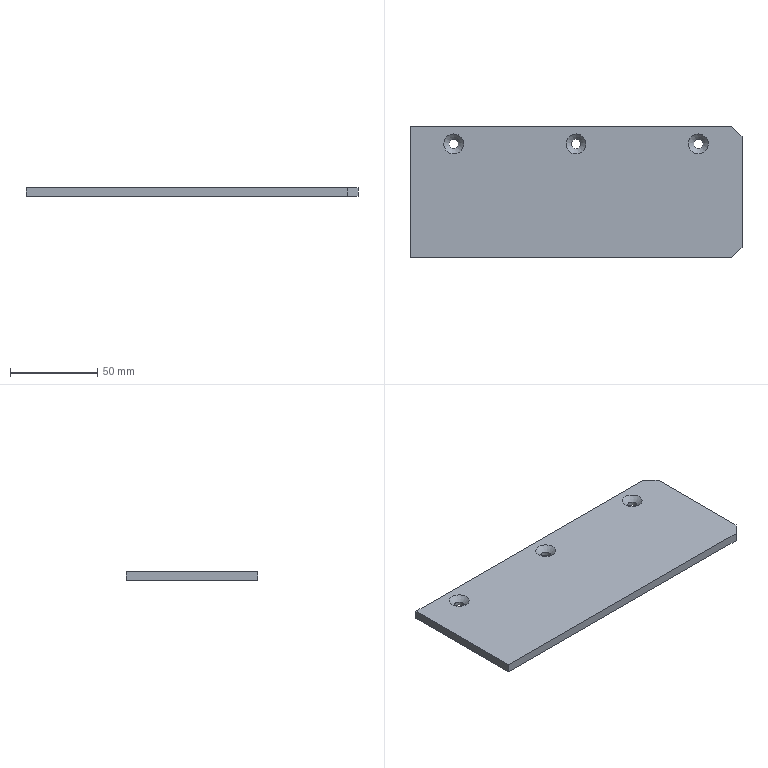Part | STEP file | P011002NF04-000 | 1 solid | 14 faces | box 190 x 75 x 5 mm | volume 70407 mm3 | plane 8 | cylinder 3 | cone 3 | commonest cylinder face diameters 5.5 x3
STEP:
#1=CARTESIAN_POINT('',(0.,0.,0.));
#2=DIRECTION('',(0.,0.,1.));
#3=DIRECTION('',(1.,0.,0.));
#4=AXIS2_PLACEMENT_3D('',#1,#2,#3);
#5=CARTESIAN_POINT('',(-107.5,200.25,265.5));
#6=VERTEX_POINT('',#5);
#7=CARTESIAN_POINT('',(-107.5,197.5,265.5));
#8=DIRECTION('',(0.,0.,1.));
#9=DIRECTION('',(0.,1.,0.));
#10=AXIS2_PLACEMENT_3D('',#7,#8,#9);
#11=CIRCLE('',#10,2.75);
#12=CARTESIAN_POINT('',(-80.,170.,265.5));
#13=DIRECTION('',(0.,0.,-1.));
#14=DIRECTION('',(-1.,0.,0.));
#15=AXIS2_PLACEMENT_3D('',#12,#13,#14);
#16=PLANE('',#15);
#17=CARTESIAN_POINT('',(27.5,30.25));
#18=CARTESIAN_POINT('',(32.263,30.25));
#19=CARTESIAN_POINT('',(29.882,26.125));
#20=CARTESIAN_POINT('',(27.5,22.));
#21=CARTESIAN_POINT('',(25.118,26.125));
#22=CARTESIAN_POINT('',(22.737,30.25));
#23=CARTESIAN_POINT('',(27.5,30.25));
#24=(BOUNDED_CURVE()B_SPLINE_CURVE(2,(#17,#18,#19,#20,#21,#22,#23),.UNSPECIFIED.,.T.,.F.)B_SPLINE_CURVE_WITH_KNOTS((1,2,2,2,2,1),(-2.094,0.,2.094,4.189,6.283,8.378),.UNSPECIFIED.)CURVE()GEOMETRIC_REPRESENTATION_ITEM()RATIONAL_B_SPLINE_CURVE((1.,0.5,1.,0.5,1.,0.5,1.))REPRESENTATION_ITEM(''));
#25=(GEOMETRIC_REPRESENTATION_CONTEXT(2)PARAMETRIC_REPRESENTATION_CONTEXT()REPRESENTATION_CONTEXT('',''));
#26=DEFINITIONAL_REPRESENTATION('',(#24),#25);
#27=PCURVE('',#16,#26);
#28=CARTESIAN_POINT('',(-107.5,197.5,267.3));
#29=DIRECTION('',(0.,0.,-1.));
#30=DIRECTION('',(0.,1.,0.));
#31=AXIS2_PLACEMENT_3D('',#28,#29,#30);
#32=CYLINDRICAL_SURFACE('',#31,2.75);
#33=CARTESIAN_POINT('',(6.283,1.8));
#34=DIRECTION('',(-1.,0.));
#35=VECTOR('',#34,1.);
#36=LINE('',#33,#35);
#37=(GEOMETRIC_REPRESENTATION_CONTEXT(2)PARAMETRIC_REPRESENTATION_CONTEXT()REPRESENTATION_CONTEXT('',''));
#38=DEFINITIONAL_REPRESENTATION('',(#36),#37);
#39=PCURVE('',#32,#38);
#40=SURFACE_CURVE('',#11,(#27,#39),.PCURVE_S1.);
#41=EDGE_CURVE('',#6,#6,#40,.T.);
#42=ORIENTED_EDGE('',*,*,#41,.T.);
#43=EDGE_LOOP('',(#42));
#44=FACE_BOUND('',#43,.T.);
#45=CARTESIAN_POINT('',(57.5,138.5,265.5));
#46=VERTEX_POINT('',#45);
#47=CARTESIAN_POINT('',(57.5,201.5,265.5));
#48=VERTEX_POINT('',#47);
#49=CARTESIAN_POINT('',(57.5,99.573,265.5));
#50=DIRECTION('',(0.,1.,0.));
#51=VECTOR('',#50,1.);
#52=LINE('',#49,#51);
#53=CARTESIAN_POINT('',(-137.5,-70.427));
#54=DIRECTION('',(0.,1.));
#55=VECTOR('',#54,1.);
#56=LINE('',#53,#55);
#57=(GEOMETRIC_REPRESENTATION_CONTEXT(2)PARAMETRIC_REPRESENTATION_CONTEXT()REPRESENTATION_CONTEXT('',''));
#58=DEFINITIONAL_REPRESENTATION('',(#56),#57);
#59=PCURVE('',#16,#58);
#60=CARTESIAN_POINT('',(57.5,99.573,271.));
#61=DIRECTION('',(1.,0.,0.));
#62=DIRECTION('',(0.,1.,0.));
#63=AXIS2_PLACEMENT_3D('',#60,#61,#62);
#64=PLANE('',#63);
#65=CARTESIAN_POINT('',(0.,-5.5));
#66=DIRECTION('',(1.,0.));
#67=VECTOR('',#66,1.);
#68=LINE('',#65,#67);
#69=(GEOMETRIC_REPRESENTATION_CONTEXT(2)PARAMETRIC_REPRESENTATION_CONTEXT()REPRESENTATION_CONTEXT('',''));
#70=DEFINITIONAL_REPRESENTATION('',(#68),#69);
#71=PCURVE('',#64,#70);
#72=SURFACE_CURVE('',#52,(#59,#71),.PCURVE_S1.);
#73=EDGE_CURVE('',#46,#48,#72,.T.);
#74=ORIENTED_EDGE('',*,*,#73,.F.);
#75=CARTESIAN_POINT('',(51.5,132.5,265.5));
#76=VERTEX_POINT('',#75);
#77=CARTESIAN_POINT('',(4.5,85.5,265.5));
#78=DIRECTION('',(-0.7071,-0.7071,0.));
#79=VECTOR('',#78,1.);
#80=LINE('',#77,#79);
#81=CARTESIAN_POINT('',(-84.5,-84.5));
#82=DIRECTION('',(0.7071,-0.7071));
#83=VECTOR('',#82,1.);
#84=LINE('',#81,#83);
#85=(GEOMETRIC_REPRESENTATION_CONTEXT(2)PARAMETRIC_REPRESENTATION_CONTEXT()REPRESENTATION_CONTEXT('',''));
#86=DEFINITIONAL_REPRESENTATION('',(#84),#85);
#87=PCURVE('',#16,#86);
#88=CARTESIAN_POINT('',(51.5,132.5,265.5));
#89=DIRECTION('',(-0.7071,0.7071,0.));
#90=DIRECTION('',(-0.7071,-0.7071,0.));
#91=AXIS2_PLACEMENT_3D('',#88,#89,#90);
#92=PLANE('',#91);
#93=CARTESIAN_POINT('',(66.468,0.));
#94=DIRECTION('',(1.,0.));
#95=VECTOR('',#94,1.);
#96=LINE('',#93,#95);
#97=(GEOMETRIC_REPRESENTATION_CONTEXT(2)PARAMETRIC_REPRESENTATION_CONTEXT()REPRESENTATION_CONTEXT('',''));
#98=DEFINITIONAL_REPRESENTATION('',(#96),#97);
#99=PCURVE('',#92,#98);
#100=SURFACE_CURVE('',#80,(#87,#99),.PCURVE_S1.);
#101=EDGE_CURVE('',#46,#76,#100,.T.);
#102=ORIENTED_EDGE('',*,*,#101,.T.);
#103=CARTESIAN_POINT('',(-132.5,132.5,265.5));
#104=VERTEX_POINT('',#103);
#105=CARTESIAN_POINT('',(-80.,132.5,265.5));
#106=DIRECTION('',(1.,0.,0.));
#107=VECTOR('',#106,1.);
#108=LINE('',#105,#107);
#109=CARTESIAN_POINT('',(0.,-37.5));
#110=DIRECTION('',(-1.,0.));
#111=VECTOR('',#110,1.);
#112=LINE('',#109,#111);
#113=(GEOMETRIC_REPRESENTATION_CONTEXT(2)PARAMETRIC_REPRESENTATION_CONTEXT()REPRESENTATION_CONTEXT('',''));
#114=DEFINITIONAL_REPRESENTATION('',(#112),#113);
#115=PCURVE('',#16,#114);
#116=CARTESIAN_POINT('',(-80.,132.5,265.5));
#117=DIRECTION('',(0.,-1.,0.));
#118=DIRECTION('',(0.,0.,-1.));
#119=AXIS2_PLACEMENT_3D('',#116,#117,#118);
#120=PLANE('',#119);
#121=CARTESIAN_POINT('',(0.,0.));
#122=DIRECTION('',(0.,1.));
#123=VECTOR('',#122,1.);
#124=LINE('',#121,#123);
#125=(GEOMETRIC_REPRESENTATION_CONTEXT(2)PARAMETRIC_REPRESENTATION_CONTEXT()REPRESENTATION_CONTEXT('',''));
#126=DEFINITIONAL_REPRESENTATION('',(#124),#125);
#127=PCURVE('',#120,#126);
#128=SURFACE_CURVE('',#108,(#115,#127),.PCURVE_S1.);
#129=EDGE_CURVE('',#104,#76,#128,.T.);
#130=ORIENTED_EDGE('',*,*,#129,.F.);
#131=CARTESIAN_POINT('',(-132.5,207.5,265.5));
#132=VERTEX_POINT('',#131);
#133=CARTESIAN_POINT('',(-132.5,295.,265.5));
#134=DIRECTION('',(0.,-1.,0.));
#135=VECTOR('',#134,1.);
#136=LINE('',#133,#135);
#137=CARTESIAN_POINT('',(52.5,125.));
#138=DIRECTION('',(0.,-1.));
#139=VECTOR('',#138,1.);
#140=LINE('',#137,#139);
#141=(GEOMETRIC_REPRESENTATION_CONTEXT(2)PARAMETRIC_REPRESENTATION_CONTEXT()REPRESENTATION_CONTEXT('',''));
#142=DEFINITIONAL_REPRESENTATION('',(#140),#141);
#143=PCURVE('',#16,#142);
#144=CARTESIAN_POINT('',(-132.5,295.,264.5));
#145=DIRECTION('',(1.,0.,0.));
#146=DIRECTION('',(0.,0.,-1.));
#147=AXIS2_PLACEMENT_3D('',#144,#145,#146);
#148=PLANE('',#147);
#149=CARTESIAN_POINT('',(-1.,0.));
#150=DIRECTION('',(0.,-1.));
#151=VECTOR('',#150,1.);
#152=LINE('',#149,#151);
#153=(GEOMETRIC_REPRESENTATION_CONTEXT(2)PARAMETRIC_REPRESENTATION_CONTEXT()REPRESENTATION_CONTEXT('',''));
#154=DEFINITIONAL_REPRESENTATION('',(#152),#153);
#155=PCURVE('',#148,#154);
#156=SURFACE_CURVE('',#136,(#143,#155),.PCURVE_S1.);
#157=EDGE_CURVE('',#132,#104,#156,.T.);
#158=ORIENTED_EDGE('',*,*,#157,.F.);
#159=CARTESIAN_POINT('',(51.5,207.5,265.5));
#160=VERTEX_POINT('',#159);
#161=CARTESIAN_POINT('',(-80.,207.5,265.5));
#162=DIRECTION('',(-1.,0.,0.));
#163=VECTOR('',#162,1.);
#164=LINE('',#161,#163);
#165=CARTESIAN_POINT('',(0.,37.5));
#166=DIRECTION('',(1.,0.));
#167=VECTOR('',#166,1.);
#168=LINE('',#165,#167);
#169=(GEOMETRIC_REPRESENTATION_CONTEXT(2)PARAMETRIC_REPRESENTATION_CONTEXT()REPRESENTATION_CONTEXT('',''));
#170=DEFINITIONAL_REPRESENTATION('',(#168),#169);
#171=PCURVE('',#16,#170);
#172=CARTESIAN_POINT('',(-80.,207.5,265.5));
#173=DIRECTION('',(0.,1.,0.));
#174=DIRECTION('',(0.,0.,1.));
#175=AXIS2_PLACEMENT_3D('',#172,#173,#174);
#176=PLANE('',#175);
#177=CARTESIAN_POINT('',(0.,0.));
#178=DIRECTION('',(0.,-1.));
#179=VECTOR('',#178,1.);
#180=LINE('',#177,#179);
#181=(GEOMETRIC_REPRESENTATION_CONTEXT(2)PARAMETRIC_REPRESENTATION_CONTEXT()REPRESENTATION_CONTEXT('',''));
#182=DEFINITIONAL_REPRESENTATION('',(#180),#181);
#183=PCURVE('',#176,#182);
#184=SURFACE_CURVE('',#164,(#171,#183),.PCURVE_S1.);
#185=EDGE_CURVE('',#160,#132,#184,.T.);
#186=ORIENTED_EDGE('',*,*,#185,.F.);
#187=CARTESIAN_POINT('',(4.5,254.5,265.5));
#188=DIRECTION('',(0.7071,-0.7071,0.));
#189=VECTOR('',#188,1.);
#190=LINE('',#187,#189);
#191=CARTESIAN_POINT('',(-84.5,84.5));
#192=DIRECTION('',(-0.7071,-0.7071));
#193=VECTOR('',#192,1.);
#194=LINE('',#191,#193);
#195=(GEOMETRIC_REPRESENTATION_CONTEXT(2)PARAMETRIC_REPRESENTATION_CONTEXT()REPRESENTATION_CONTEXT('',''));
#196=DEFINITIONAL_REPRESENTATION('',(#194),#195);
#197=PCURVE('',#16,#196);
#198=CARTESIAN_POINT('',(57.5,201.5,271.));
#199=DIRECTION('',(-0.7071,-0.7071,0.));
#200=DIRECTION('',(0.7071,-0.7071,0.));
#201=AXIS2_PLACEMENT_3D('',#198,#199,#200);
#202=PLANE('',#201);
#203=CARTESIAN_POINT('',(-74.953,-5.5));
#204=DIRECTION('',(1.,0.));
#205=VECTOR('',#204,1.);
#206=LINE('',#203,#205);
#207=(GEOMETRIC_REPRESENTATION_CONTEXT(2)PARAMETRIC_REPRESENTATION_CONTEXT()REPRESENTATION_CONTEXT('',''));
#208=DEFINITIONAL_REPRESENTATION('',(#206),#207);
#209=PCURVE('',#202,#208);
#210=SURFACE_CURVE('',#190,(#197,#209),.PCURVE_S1.);
#211=EDGE_CURVE('',#160,#48,#210,.T.);
#212=ORIENTED_EDGE('',*,*,#211,.T.);
#213=EDGE_LOOP('',(#74,#102,#130,#158,#186,#212));
#214=FACE_BOUND('',#213,.T.);
#215=CARTESIAN_POINT('',(-37.5,200.25,265.5));
#216=VERTEX_POINT('',#215);
#217=CARTESIAN_POINT('',(-37.5,197.5,265.5));
#218=DIRECTION('',(0.,0.,1.));
#219=DIRECTION('',(0.,1.,0.));
#220=AXIS2_PLACEMENT_3D('',#217,#218,#219);
#221=CIRCLE('',#220,2.75);
#222=CARTESIAN_POINT('',(-42.5,30.25));
#223=CARTESIAN_POINT('',(-37.737,30.25));
#224=CARTESIAN_POINT('',(-40.118,26.125));
#225=CARTESIAN_POINT('',(-42.5,22.));
#226=CARTESIAN_POINT('',(-44.882,26.125));
#227=CARTESIAN_POINT('',(-47.263,30.25));
#228=CARTESIAN_POINT('',(-42.5,30.25));
#229=(BOUNDED_CURVE()B_SPLINE_CURVE(2,(#222,#223,#224,#225,#226,#227,#228),.UNSPECIFIED.,.T.,.F.)B_SPLINE_CURVE_WITH_KNOTS((1,2,2,2,2,1),(-2.094,0.,2.094,4.189,6.283,8.378),.UNSPECIFIED.)CURVE()GEOMETRIC_REPRESENTATION_ITEM()RATIONAL_B_SPLINE_CURVE((1.,0.5,1.,0.5,1.,0.5,1.))REPRESENTATION_ITEM(''));
#230=(GEOMETRIC_REPRESENTATION_CONTEXT(2)PARAMETRIC_REPRESENTATION_CONTEXT()REPRESENTATION_CONTEXT('',''));
#231=DEFINITIONAL_REPRESENTATION('',(#229),#230);
#232=PCURVE('',#16,#231);
#233=CARTESIAN_POINT('',(-37.5,197.5,267.3));
#234=DIRECTION('',(0.,0.,-1.));
#235=DIRECTION('',(0.,1.,0.));
#236=AXIS2_PLACEMENT_3D('',#233,#234,#235);
#237=CYLINDRICAL_SURFACE('',#236,2.75);
#238=CARTESIAN_POINT('',(6.283,1.8));
#239=DIRECTION('',(-1.,0.));
#240=VECTOR('',#239,1.);
#241=LINE('',#238,#240);
#242=(GEOMETRIC_REPRESENTATION_CONTEXT(2)PARAMETRIC_REPRESENTATION_CONTEXT()REPRESENTATION_CONTEXT('',''));
#243=DEFINITIONAL_REPRESENTATION('',(#241),#242);
#244=PCURVE('',#237,#243);
#245=SURFACE_CURVE('',#221,(#232,#244),.PCURVE_S1.);
#246=EDGE_CURVE('',#216,#216,#245,.T.);
#247=ORIENTED_EDGE('',*,*,#246,.T.);
#248=EDGE_LOOP('',(#247));
#249=FACE_BOUND('',#248,.T.);
#250=CARTESIAN_POINT('',(32.5,200.25,265.5));
#251=VERTEX_POINT('',#250);
#252=CARTESIAN_POINT('',(32.5,197.5,265.5));
#253=DIRECTION('',(0.,0.,1.));
#254=DIRECTION('',(0.,1.,0.));
#255=AXIS2_PLACEMENT_3D('',#252,#253,#254);
#256=CIRCLE('',#255,2.75);
#257=CARTESIAN_POINT('',(-112.5,30.25));
#258=CARTESIAN_POINT('',(-107.737,30.25));
#259=CARTESIAN_POINT('',(-110.118,26.125));
#260=CARTESIAN_POINT('',(-112.5,22.));
#261=CARTESIAN_POINT('',(-114.882,26.125));
#262=CARTESIAN_POINT('',(-117.263,30.25));
#263=CARTESIAN_POINT('',(-112.5,30.25));
#264=(BOUNDED_CURVE()B_SPLINE_CURVE(2,(#257,#258,#259,#260,#261,#262,#263),.UNSPECIFIED.,.T.,.F.)B_SPLINE_CURVE_WITH_KNOTS((1,2,2,2,2,1),(-2.094,0.,2.094,4.189,6.283,8.378),.UNSPECIFIED.)CURVE()GEOMETRIC_REPRESENTATION_ITEM()RATIONAL_B_SPLINE_CURVE((1.,0.5,1.,0.5,1.,0.5,1.))REPRESENTATION_ITEM(''));
#265=(GEOMETRIC_REPRESENTATION_CONTEXT(2)PARAMETRIC_REPRESENTATION_CONTEXT()REPRESENTATION_CONTEXT('',''));
#266=DEFINITIONAL_REPRESENTATION('',(#264),#265);
#267=PCURVE('',#16,#266);
#268=CARTESIAN_POINT('',(32.5,197.5,267.3));
#269=DIRECTION('',(0.,0.,-1.));
#270=DIRECTION('',(0.,1.,0.));
#271=AXIS2_PLACEMENT_3D('',#268,#269,#270);
#272=CYLINDRICAL_SURFACE('',#271,2.75);
#273=CARTESIAN_POINT('',(6.283,1.8));
#274=DIRECTION('',(-1.,0.));
#275=VECTOR('',#274,1.);
#276=LINE('',#273,#275);
#277=(GEOMETRIC_REPRESENTATION_CONTEXT(2)PARAMETRIC_REPRESENTATION_CONTEXT()REPRESENTATION_CONTEXT('',''));
#278=DEFINITIONAL_REPRESENTATION('',(#276),#277);
#279=PCURVE('',#272,#278);
#280=SURFACE_CURVE('',#256,(#267,#279),.PCURVE_S1.);
#281=EDGE_CURVE('',#251,#251,#280,.T.);
#282=ORIENTED_EDGE('',*,*,#281,.T.);
#283=EDGE_LOOP('',(#282));
#284=FACE_BOUND('',#283,.T.);
#285=ADVANCED_FACE('',(#44,#214,#249,#284),#16,.T.);
#286=CARTESIAN_POINT('',(38.2,197.5,270.5));
#287=VERTEX_POINT('',#286);
#288=CARTESIAN_POINT('',(32.5,203.2,270.5));
#289=VERTEX_POINT('',#288);
#290=CARTESIAN_POINT('',(32.5,197.5,270.5));
#291=DIRECTION('',(0.,0.,1.));
#292=DIRECTION('',(1.,0.,0.));
#293=AXIS2_PLACEMENT_3D('',#290,#291,#292);
#294=CIRCLE('',#293,5.7);
#295=CARTESIAN_POINT('',(-80.,170.,270.5));
#296=DIRECTION('',(0.,0.,1.));
#297=DIRECTION('',(1.,0.,0.));
#298=AXIS2_PLACEMENT_3D('',#295,#296,#297);
#299=PLANE('',#298);
#300=CARTESIAN_POINT('',(112.5,27.5));
#301=DIRECTION('',(1.,0.));
#302=AXIS2_PLACEMENT_2D('',#300,#301);
#303=CIRCLE('',#302,5.7);
#304=(GEOMETRIC_REPRESENTATION_CONTEXT(2)PARAMETRIC_REPRESENTATION_CONTEXT()REPRESENTATION_CONTEXT('',''));
#305=DEFINITIONAL_REPRESENTATION('',(#303),#304);
#306=PCURVE('',#299,#305);
#307=CARTESIAN_POINT('',(32.5,197.5,267.3));
#308=DIRECTION('',(0.,0.,1.));
#309=DIRECTION('',(0.,1.,0.));
#310=AXIS2_PLACEMENT_3D('',#307,#308,#309);
#311=CONICAL_SURFACE('',#310,2.5,0.7854);
#312=CARTESIAN_POINT('',(4.712,3.2));
#313=DIRECTION('',(1.,0.));
#314=VECTOR('',#313,1.);
#315=LINE('',#312,#314);
#316=(GEOMETRIC_REPRESENTATION_CONTEXT(2)PARAMETRIC_REPRESENTATION_CONTEXT()REPRESENTATION_CONTEXT('',''));
#317=DEFINITIONAL_REPRESENTATION('',(#315),#316);
#318=PCURVE('',#311,#317);
#319=SURFACE_CURVE('',#294,(#306,#318),.PCURVE_S1.);
#320=EDGE_CURVE('',#287,#289,#319,.T.);
#321=ORIENTED_EDGE('',*,*,#320,.F.);
#322=CARTESIAN_POINT('',(32.5,197.5,270.5));
#323=DIRECTION('',(0.,0.,1.));
#324=DIRECTION('',(1.,0.,0.));
#325=AXIS2_PLACEMENT_3D('',#322,#323,#324);
#326=CIRCLE('',#325,5.7);
#327=CARTESIAN_POINT('',(112.5,27.5));
#328=DIRECTION('',(1.,0.));
#329=AXIS2_PLACEMENT_2D('',#327,#328);
#330=CIRCLE('',#329,5.7);
#331=(GEOMETRIC_REPRESENTATION_CONTEXT(2)PARAMETRIC_REPRESENTATION_CONTEXT()REPRESENTATION_CONTEXT('',''));
#332=DEFINITIONAL_REPRESENTATION('',(#330),#331);
#333=PCURVE('',#299,#332);
#334=CARTESIAN_POINT('',(-1.571,3.2));
#335=DIRECTION('',(1.,0.));
#336=VECTOR('',#335,1.);
#337=LINE('',#334,#336);
#338=(GEOMETRIC_REPRESENTATION_CONTEXT(2)PARAMETRIC_REPRESENTATION_CONTEXT()REPRESENTATION_CONTEXT('',''));
#339=DEFINITIONAL_REPRESENTATION('',(#337),#338);
#340=PCURVE('',#311,#339);
#341=SURFACE_CURVE('',#326,(#333,#340),.PCURVE_S1.);
#342=EDGE_CURVE('',#289,#287,#341,.T.);
#343=ORIENTED_EDGE('',*,*,#342,.F.);
#344=EDGE_LOOP('',(#321,#343));
#345=FACE_BOUND('',#344,.T.);
#346=CARTESIAN_POINT('',(-101.8,197.5,270.5));
#347=VERTEX_POINT('',#346);
#348=CARTESIAN_POINT('',(-107.5,203.2,270.5));
#349=VERTEX_POINT('',#348);
#350=CARTESIAN_POINT('',(-107.5,197.5,270.5));
#351=DIRECTION('',(0.,0.,1.));
#352=DIRECTION('',(1.,0.,0.));
#353=AXIS2_PLACEMENT_3D('',#350,#351,#352);
#354=CIRCLE('',#353,5.7);
#355=CARTESIAN_POINT('',(-27.5,27.5));
#356=DIRECTION('',(1.,0.));
#357=AXIS2_PLACEMENT_2D('',#355,#356);
#358=CIRCLE('',#357,5.7);
#359=(GEOMETRIC_REPRESENTATION_CONTEXT(2)PARAMETRIC_REPRESENTATION_CONTEXT()REPRESENTATION_CONTEXT('',''));
#360=DEFINITIONAL_REPRESENTATION('',(#358),#359);
#361=PCURVE('',#299,#360);
#362=CARTESIAN_POINT('',(-107.5,197.5,267.3));
#363=DIRECTION('',(0.,0.,1.));
#364=DIRECTION('',(0.,1.,0.));
#365=AXIS2_PLACEMENT_3D('',#362,#363,#364);
#366=CONICAL_SURFACE('',#365,2.5,0.7854);
#367=CARTESIAN_POINT('',(4.712,3.2));
#368=DIRECTION('',(1.,0.));
#369=VECTOR('',#368,1.);
#370=LINE('',#367,#369);
#371=(GEOMETRIC_REPRESENTATION_CONTEXT(2)PARAMETRIC_REPRESENTATION_CONTEXT()REPRESENTATION_CONTEXT('',''));
#372=DEFINITIONAL_REPRESENTATION('',(#370),#371);
#373=PCURVE('',#366,#372);
#374=SURFACE_CURVE('',#354,(#361,#373),.PCURVE_S1.);
#375=EDGE_CURVE('',#347,#349,#374,.T.);
#376=ORIENTED_EDGE('',*,*,#375,.F.);
#377=CARTESIAN_POINT('',(-107.5,197.5,270.5));
#378=DIRECTION('',(0.,0.,1.));
#379=DIRECTION('',(1.,0.,0.));
#380=AXIS2_PLACEMENT_3D('',#377,#378,#379);
#381=CIRCLE('',#380,5.7);
#382=CARTESIAN_POINT('',(-27.5,27.5));
#383=DIRECTION('',(1.,0.));
#384=AXIS2_PLACEMENT_2D('',#382,#383);
#385=CIRCLE('',#384,5.7);
#386=(GEOMETRIC_REPRESENTATION_CONTEXT(2)PARAMETRIC_REPRESENTATION_CONTEXT()REPRESENTATION_CONTEXT('',''));
#387=DEFINITIONAL_REPRESENTATION('',(#385),#386);
#388=PCURVE('',#299,#387);
#389=CARTESIAN_POINT('',(-1.571,3.2));
#390=DIRECTION('',(1.,0.));
#391=VECTOR('',#390,1.);
#392=LINE('',#389,#391);
#393=(GEOMETRIC_REPRESENTATION_CONTEXT(2)PARAMETRIC_REPRESENTATION_CONTEXT()REPRESENTATION_CONTEXT('',''));
#394=DEFINITIONAL_REPRESENTATION('',(#392),#393);
#395=PCURVE('',#366,#394);
#396=SURFACE_CURVE('',#381,(#388,#395),.PCURVE_S1.);
#397=EDGE_CURVE('',#349,#347,#396,.T.);
#398=ORIENTED_EDGE('',*,*,#397,.F.);
#399=EDGE_LOOP('',(#376,#398));
#400=FACE_BOUND('',#399,.T.);
#401=CARTESIAN_POINT('',(-31.8,197.5,270.5));
#402=VERTEX_POINT('',#401);
#403=CARTESIAN_POINT('',(-37.5,203.2,270.5));
#404=VERTEX_POINT('',#403);
#405=CARTESIAN_POINT('',(-37.5,197.5,270.5));
#406=DIRECTION('',(0.,0.,1.));
#407=DIRECTION('',(1.,0.,0.));
#408=AXIS2_PLACEMENT_3D('',#405,#406,#407);
#409=CIRCLE('',#408,5.7);
#410=CARTESIAN_POINT('',(42.5,27.5));
#411=DIRECTION('',(1.,0.));
#412=AXIS2_PLACEMENT_2D('',#410,#411);
#413=CIRCLE('',#412,5.7);
#414=(GEOMETRIC_REPRESENTATION_CONTEXT(2)PARAMETRIC_REPRESENTATION_CONTEXT()REPRESENTATION_CONTEXT('',''));
#415=DEFINITIONAL_REPRESENTATION('',(#413),#414);
#416=PCURVE('',#299,#415);
#417=CARTESIAN_POINT('',(-37.5,197.5,267.3));
#418=DIRECTION('',(0.,0.,1.));
#419=DIRECTION('',(0.,1.,0.));
#420=AXIS2_PLACEMENT_3D('',#417,#418,#419);
#421=CONICAL_SURFACE('',#420,2.5,0.7854);
#422=CARTESIAN_POINT('',(4.712,3.2));
#423=DIRECTION('',(1.,0.));
#424=VECTOR('',#423,1.);
#425=LINE('',#422,#424);
#426=(GEOMETRIC_REPRESENTATION_CONTEXT(2)PARAMETRIC_REPRESENTATION_CONTEXT()REPRESENTATION_CONTEXT('',''));
#427=DEFINITIONAL_REPRESENTATION('',(#425),#426);
#428=PCURVE('',#421,#427);
#429=SURFACE_CURVE('',#409,(#416,#428),.PCURVE_S1.);
#430=EDGE_CURVE('',#402,#404,#429,.T.);
#431=ORIENTED_EDGE('',*,*,#430,.F.);
#432=CARTESIAN_POINT('',(-37.5,197.5,270.5));
#433=DIRECTION('',(0.,0.,1.));
#434=DIRECTION('',(1.,0.,0.));
#435=AXIS2_PLACEMENT_3D('',#432,#433,#434);
#436=CIRCLE('',#435,5.7);
#437=CARTESIAN_POINT('',(42.5,27.5));
#438=DIRECTION('',(1.,0.));
#439=AXIS2_PLACEMENT_2D('',#437,#438);
#440=CIRCLE('',#439,5.7);
#441=(GEOMETRIC_REPRESENTATION_CONTEXT(2)PARAMETRIC_REPRESENTATION_CONTEXT()REPRESENTATION_CONTEXT('',''));
#442=DEFINITIONAL_REPRESENTATION('',(#440),#441);
#443=PCURVE('',#299,#442);
#444=CARTESIAN_POINT('',(-1.571,3.2));
#445=DIRECTION('',(1.,0.));
#446=VECTOR('',#445,1.);
#447=LINE('',#444,#446);
#448=(GEOMETRIC_REPRESENTATION_CONTEXT(2)PARAMETRIC_REPRESENTATION_CONTEXT()REPRESENTATION_CONTEXT('',''));
#449=DEFINITIONAL_REPRESENTATION('',(#447),#448);
#450=PCURVE('',#421,#449);
#451=SURFACE_CURVE('',#436,(#443,#450),.PCURVE_S1.);
#452=EDGE_CURVE('',#404,#402,#451,.T.);
#453=ORIENTED_EDGE('',*,*,#452,.F.);
#454=EDGE_LOOP('',(#431,#453));
#455=FACE_BOUND('',#454,.T.);
#456=CARTESIAN_POINT('',(51.5,132.5,270.5));
#457=VERTEX_POINT('',#456);
#458=CARTESIAN_POINT('',(-132.5,132.5,270.5));
#459=VERTEX_POINT('',#458);
#460=CARTESIAN_POINT('',(-80.,132.5,270.5));
#461=DIRECTION('',(-1.,0.,0.));
#462=VECTOR('',#461,1.);
#463=LINE('',#460,#462);
#464=CARTESIAN_POINT('',(0.,-37.5));
#465=DIRECTION('',(-1.,0.));
#466=VECTOR('',#465,1.);
#467=LINE('',#464,#466);
#468=(GEOMETRIC_REPRESENTATION_CONTEXT(2)PARAMETRIC_REPRESENTATION_CONTEXT()REPRESENTATION_CONTEXT('',''));
#469=DEFINITIONAL_REPRESENTATION('',(#467),#468);
#470=PCURVE('',#299,#469);
#471=CARTESIAN_POINT('',(-5.,0.));
#472=DIRECTION('',(0.,-1.));
#473=VECTOR('',#472,1.);
#474=LINE('',#471,#473);
#475=(GEOMETRIC_REPRESENTATION_CONTEXT(2)PARAMETRIC_REPRESENTATION_CONTEXT()REPRESENTATION_CONTEXT('',''));
#476=DEFINITIONAL_REPRESENTATION('',(#474),#475);
#477=PCURVE('',#120,#476);
#478=SURFACE_CURVE('',#463,(#470,#477),.PCURVE_S1.);
#479=EDGE_CURVE('',#457,#459,#478,.T.);
#480=ORIENTED_EDGE('',*,*,#479,.F.);
#481=CARTESIAN_POINT('',(57.5,138.5,270.5));
#482=VERTEX_POINT('',#481);
#483=CARTESIAN_POINT('',(4.5,85.5,270.5));
#484=DIRECTION('',(0.7071,0.7071,0.));
#485=VECTOR('',#484,1.);
#486=LINE('',#483,#485);
#487=CARTESIAN_POINT('',(84.5,-84.5));
#488=DIRECTION('',(0.7071,0.7071));
#489=VECTOR('',#488,1.);
#490=LINE('',#487,#489);
#491=(GEOMETRIC_REPRESENTATION_CONTEXT(2)PARAMETRIC_REPRESENTATION_CONTEXT()REPRESENTATION_CONTEXT('',''));
#492=DEFINITIONAL_REPRESENTATION('',(#490),#491);
#493=PCURVE('',#299,#492);
#494=CARTESIAN_POINT('',(66.468,5.));
#495=DIRECTION('',(-1.,0.));
#496=VECTOR('',#495,1.);
#497=LINE('',#494,#496);
#498=(GEOMETRIC_REPRESENTATION_CONTEXT(2)PARAMETRIC_REPRESENTATION_CONTEXT()REPRESENTATION_CONTEXT('',''));
#499=DEFINITIONAL_REPRESENTATION('',(#497),#498);
#500=PCURVE('',#92,#499);
#501=SURFACE_CURVE('',#486,(#493,#500),.PCURVE_S1.);
#502=EDGE_CURVE('',#457,#482,#501,.T.);
#503=ORIENTED_EDGE('',*,*,#502,.T.);
#504=CARTESIAN_POINT('',(57.5,201.5,270.5));
#505=VERTEX_POINT('',#504);
#506=CARTESIAN_POINT('',(57.5,99.573,270.5));
#507=DIRECTION('',(0.,-1.,0.));
#508=VECTOR('',#507,1.);
#509=LINE('',#506,#508);
#510=CARTESIAN_POINT('',(137.5,-70.427));
#511=DIRECTION('',(0.,-1.));
#512=VECTOR('',#511,1.);
#513=LINE('',#510,#512);
#514=(GEOMETRIC_REPRESENTATION_CONTEXT(2)PARAMETRIC_REPRESENTATION_CONTEXT()REPRESENTATION_CONTEXT('',''));
#515=DEFINITIONAL_REPRESENTATION('',(#513),#514);
#516=PCURVE('',#299,#515);
#517=CARTESIAN_POINT('',(0.,-0.5));
#518=DIRECTION('',(-1.,0.));
#519=VECTOR('',#518,1.);
#520=LINE('',#517,#519);
#521=(GEOMETRIC_REPRESENTATION_CONTEXT(2)PARAMETRIC_REPRESENTATION_CONTEXT()REPRESENTATION_CONTEXT('',''));
#522=DEFINITIONAL_REPRESENTATION('',(#520),#521);
#523=PCURVE('',#64,#522);
#524=SURFACE_CURVE('',#509,(#516,#523),.PCURVE_S1.);
#525=EDGE_CURVE('',#505,#482,#524,.T.);
#526=ORIENTED_EDGE('',*,*,#525,.F.);
#527=CARTESIAN_POINT('',(51.5,207.5,270.5));
#528=VERTEX_POINT('',#527);
#529=CARTESIAN_POINT('',(4.5,254.5,270.5));
#530=DIRECTION('',(-0.7071,0.7071,0.));
#531=VECTOR('',#530,1.);
#532=LINE('',#529,#531);
#533=CARTESIAN_POINT('',(84.5,84.5));
#534=DIRECTION('',(-0.7071,0.7071));
#535=VECTOR('',#534,1.);
#536=LINE('',#533,#535);
#537=(GEOMETRIC_REPRESENTATION_CONTEXT(2)PARAMETRIC_REPRESENTATION_CONTEXT()REPRESENTATION_CONTEXT('',''));
#538=DEFINITIONAL_REPRESENTATION('',(#536),#537);
#539=PCURVE('',#299,#538);
#540=CARTESIAN_POINT('',(-74.953,-0.5));
#541=DIRECTION('',(-1.,0.));
#542=VECTOR('',#541,1.);
#543=LINE('',#540,#542);
#544=(GEOMETRIC_REPRESENTATION_CONTEXT(2)PARAMETRIC_REPRESENTATION_CONTEXT()REPRESENTATION_CONTEXT('',''));
#545=DEFINITIONAL_REPRESENTATION('',(#543),#544);
#546=PCURVE('',#202,#545);
#547=SURFACE_CURVE('',#532,(#539,#546),.PCURVE_S1.);
#548=EDGE_CURVE('',#505,#528,#547,.T.);
#549=ORIENTED_EDGE('',*,*,#548,.T.);
#550=CARTESIAN_POINT('',(-132.5,207.5,270.5));
#551=VERTEX_POINT('',#550);
#552=CARTESIAN_POINT('',(-80.,207.5,270.5));
#553=DIRECTION('',(1.,0.,0.));
#554=VECTOR('',#553,1.);
#555=LINE('',#552,#554);
#556=CARTESIAN_POINT('',(0.,37.5));
#557=DIRECTION('',(1.,0.));
#558=VECTOR('',#557,1.);
#559=LINE('',#556,#558);
#560=(GEOMETRIC_REPRESENTATION_CONTEXT(2)PARAMETRIC_REPRESENTATION_CONTEXT()REPRESENTATION_CONTEXT('',''));
#561=DEFINITIONAL_REPRESENTATION('',(#559),#560);
#562=PCURVE('',#299,#561);
#563=CARTESIAN_POINT('',(5.,0.));
#564=DIRECTION('',(0.,1.));
#565=VECTOR('',#564,1.);
#566=LINE('',#563,#565);
#567=(GEOMETRIC_REPRESENTATION_CONTEXT(2)PARAMETRIC_REPRESENTATION_CONTEXT()REPRESENTATION_CONTEXT('',''));
#568=DEFINITIONAL_REPRESENTATION('',(#566),#567);
#569=PCURVE('',#176,#568);
#570=SURFACE_CURVE('',#555,(#562,#569),.PCURVE_S1.);
#571=EDGE_CURVE('',#551,#528,#570,.T.);
#572=ORIENTED_EDGE('',*,*,#571,.F.);
#573=CARTESIAN_POINT('',(-132.5,295.,270.5));
#574=DIRECTION('',(0.,1.,0.));
#575=VECTOR('',#574,1.);
#576=LINE('',#573,#575);
#577=CARTESIAN_POINT('',(-52.5,125.));
#578=DIRECTION('',(0.,1.));
#579=VECTOR('',#578,1.);
#580=LINE('',#577,#579);
#581=(GEOMETRIC_REPRESENTATION_CONTEXT(2)PARAMETRIC_REPRESENTATION_CONTEXT()REPRESENTATION_CONTEXT('',''));
#582=DEFINITIONAL_REPRESENTATION('',(#580),#581);
#583=PCURVE('',#299,#582);
#584=CARTESIAN_POINT('',(-6.,0.));
#585=DIRECTION('',(0.,1.));
#586=VECTOR('',#585,1.);
#587=LINE('',#584,#586);
#588=(GEOMETRIC_REPRESENTATION_CONTEXT(2)PARAMETRIC_REPRESENTATION_CONTEXT()REPRESENTATION_CONTEXT('',''));
#589=DEFINITIONAL_REPRESENTATION('',(#587),#588);
#590=PCURVE('',#148,#589);
#591=SURFACE_CURVE('',#576,(#583,#590),.PCURVE_S1.);
#592=EDGE_CURVE('',#459,#551,#591,.T.);
#593=ORIENTED_EDGE('',*,*,#592,.F.);
#594=EDGE_LOOP('',(#480,#503,#526,#549,#572,#593));
#595=FACE_BOUND('',#594,.T.);
#596=ADVANCED_FACE('',(#345,#400,#455,#595),#299,.T.);
#597=ORIENTED_EDGE('',*,*,#129,.T.);
#598=CARTESIAN_POINT('',(51.5,132.5,265.5));
#599=DIRECTION('',(0.,0.,1.));
#600=VECTOR('',#599,1.);
#601=LINE('',#598,#600);
#602=CARTESIAN_POINT('',(0.,131.5));
#603=DIRECTION('',(-1.,0.));
#604=VECTOR('',#603,1.);
#605=LINE('',#602,#604);
#606=(GEOMETRIC_REPRESENTATION_CONTEXT(2)PARAMETRIC_REPRESENTATION_CONTEXT()REPRESENTATION_CONTEXT('',''));
#607=DEFINITIONAL_REPRESENTATION('',(#605),#606);
#608=PCURVE('',#120,#607);
#609=CARTESIAN_POINT('',(0.,0.));
#610=DIRECTION('',(0.,1.));
#611=VECTOR('',#610,1.);
#612=LINE('',#609,#611);
#613=(GEOMETRIC_REPRESENTATION_CONTEXT(2)PARAMETRIC_REPRESENTATION_CONTEXT()REPRESENTATION_CONTEXT('',''));
#614=DEFINITIONAL_REPRESENTATION('',(#612),#613);
#615=PCURVE('',#92,#614);
#616=SURFACE_CURVE('',#601,(#608,#615),.PCURVE_S1.);
#617=EDGE_CURVE('',#76,#457,#616,.T.);
#618=ORIENTED_EDGE('',*,*,#617,.T.);
#619=ORIENTED_EDGE('',*,*,#479,.T.);
#620=CARTESIAN_POINT('',(-132.5,132.5,264.5));
#621=DIRECTION('',(0.,0.,1.));
#622=VECTOR('',#621,1.);
#623=LINE('',#620,#622);
#624=CARTESIAN_POINT('',(1.,-52.5));
#625=DIRECTION('',(-1.,0.));
#626=VECTOR('',#625,1.);
#627=LINE('',#624,#626);
#628=(GEOMETRIC_REPRESENTATION_CONTEXT(2)PARAMETRIC_REPRESENTATION_CONTEXT()REPRESENTATION_CONTEXT('',''));
#629=DEFINITIONAL_REPRESENTATION('',(#627),#628);
#630=PCURVE('',#120,#629);
#631=CARTESIAN_POINT('',(0.,-162.5));
#632=DIRECTION('',(-1.,0.));
#633=VECTOR('',#632,1.);
#634=LINE('',#631,#633);
#635=(GEOMETRIC_REPRESENTATION_CONTEXT(2)PARAMETRIC_REPRESENTATION_CONTEXT()REPRESENTATION_CONTEXT('',''));
#636=DEFINITIONAL_REPRESENTATION('',(#634),#635);
#637=PCURVE('',#148,#636);
#638=SURFACE_CURVE('',#623,(#630,#637),.PCURVE_S1.);
#639=EDGE_CURVE('',#104,#459,#638,.T.);
#640=ORIENTED_EDGE('',*,*,#639,.F.);
#641=EDGE_LOOP('',(#597,#618,#619,#640));
#642=FACE_BOUND('',#641,.T.);
#643=ADVANCED_FACE('',(#642),#120,.T.);
#644=ORIENTED_EDGE('',*,*,#639,.T.);
#645=ORIENTED_EDGE('',*,*,#592,.T.);
#646=CARTESIAN_POINT('',(-132.5,207.5,265.5));
#647=DIRECTION('',(0.,0.,1.));
#648=VECTOR('',#647,1.);
#649=LINE('',#646,#648);
#650=CARTESIAN_POINT('',(-1.,-87.5));
#651=DIRECTION('',(-1.,0.));
#652=VECTOR('',#651,1.);
#653=LINE('',#650,#652);
#654=(GEOMETRIC_REPRESENTATION_CONTEXT(2)PARAMETRIC_REPRESENTATION_CONTEXT()REPRESENTATION_CONTEXT('',''));
#655=DEFINITIONAL_REPRESENTATION('',(#653),#654);
#656=PCURVE('',#148,#655);
#657=CARTESIAN_POINT('',(0.,-52.5));
#658=DIRECTION('',(1.,0.));
#659=VECTOR('',#658,1.);
#660=LINE('',#657,#659);
#661=(GEOMETRIC_REPRESENTATION_CONTEXT(2)PARAMETRIC_REPRESENTATION_CONTEXT()REPRESENTATION_CONTEXT('',''));
#662=DEFINITIONAL_REPRESENTATION('',(#660),#661);
#663=PCURVE('',#176,#662);
#664=SURFACE_CURVE('',#649,(#656,#663),.PCURVE_S1.);
#665=EDGE_CURVE('',#132,#551,#664,.T.);
#666=ORIENTED_EDGE('',*,*,#665,.F.);
#667=ORIENTED_EDGE('',*,*,#157,.T.);
#668=EDGE_LOOP('',(#644,#645,#666,#667));
#669=FACE_BOUND('',#668,.T.);
#670=ADVANCED_FACE('',(#669),#148,.F.);
#671=ORIENTED_EDGE('',*,*,#571,.T.);
#672=CARTESIAN_POINT('',(51.5,207.5,265.5));
#673=DIRECTION('',(0.,0.,-1.));
#674=VECTOR('',#673,1.);
#675=LINE('',#672,#674);
#676=CARTESIAN_POINT('',(0.,131.5));
#677=DIRECTION('',(-1.,0.));
#678=VECTOR('',#677,1.);
#679=LINE('',#676,#678);
#680=(GEOMETRIC_REPRESENTATION_CONTEXT(2)PARAMETRIC_REPRESENTATION_CONTEXT()REPRESENTATION_CONTEXT('',''));
#681=DEFINITIONAL_REPRESENTATION('',(#679),#680);
#682=PCURVE('',#176,#681);
#683=CARTESIAN_POINT('',(-8.485,-5.5));
#684=DIRECTION('',(0.,-1.));
#685=VECTOR('',#684,1.);
#686=LINE('',#683,#685);
#687=(GEOMETRIC_REPRESENTATION_CONTEXT(2)PARAMETRIC_REPRESENTATION_CONTEXT()REPRESENTATION_CONTEXT('',''));
#688=DEFINITIONAL_REPRESENTATION('',(#686),#687);
#689=PCURVE('',#202,#688);
#690=SURFACE_CURVE('',#675,(#682,#689),.PCURVE_S1.);
#691=EDGE_CURVE('',#528,#160,#690,.T.);
#692=ORIENTED_EDGE('',*,*,#691,.T.);
#693=ORIENTED_EDGE('',*,*,#185,.T.);
#694=ORIENTED_EDGE('',*,*,#665,.T.);
#695=EDGE_LOOP('',(#671,#692,#693,#694));
#696=FACE_BOUND('',#695,.T.);
#697=ADVANCED_FACE('',(#696),#176,.T.);
#698=ORIENTED_EDGE('',*,*,#525,.T.);
#699=CARTESIAN_POINT('',(57.5,138.5,271.));
#700=DIRECTION('',(0.,0.,-1.));
#701=VECTOR('',#700,1.);
#702=LINE('',#699,#701);
#703=CARTESIAN_POINT('',(38.927,0.));
#704=DIRECTION('',(0.,-1.));
#705=VECTOR('',#704,1.);
#706=LINE('',#703,#705);
#707=(GEOMETRIC_REPRESENTATION_CONTEXT(2)PARAMETRIC_REPRESENTATION_CONTEXT()REPRESENTATION_CONTEXT('',''));
#708=DEFINITIONAL_REPRESENTATION('',(#706),#707);
#709=PCURVE('',#64,#708);
#710=CARTESIAN_POINT('',(-8.485,5.5));
#711=DIRECTION('',(0.,-1.));
#712=VECTOR('',#711,1.);
#713=LINE('',#710,#712);
#714=(GEOMETRIC_REPRESENTATION_CONTEXT(2)PARAMETRIC_REPRESENTATION_CONTEXT()REPRESENTATION_CONTEXT('',''));
#715=DEFINITIONAL_REPRESENTATION('',(#713),#714);
#716=PCURVE('',#92,#715);
#717=SURFACE_CURVE('',#702,(#709,#716),.PCURVE_S1.);
#718=EDGE_CURVE('',#482,#46,#717,.T.);
#719=ORIENTED_EDGE('',*,*,#718,.T.);
#720=ORIENTED_EDGE('',*,*,#73,.T.);
#721=CARTESIAN_POINT('',(57.5,201.5,271.));
#722=DIRECTION('',(0.,0.,1.));
#723=VECTOR('',#722,1.);
#724=LINE('',#721,#723);
#725=CARTESIAN_POINT('',(101.927,0.));
#726=DIRECTION('',(0.,1.));
#727=VECTOR('',#726,1.);
#728=LINE('',#725,#727);
#729=(GEOMETRIC_REPRESENTATION_CONTEXT(2)PARAMETRIC_REPRESENTATION_CONTEXT()REPRESENTATION_CONTEXT('',''));
#730=DEFINITIONAL_REPRESENTATION('',(#728),#729);
#731=PCURVE('',#64,#730);
#732=CARTESIAN_POINT('',(0.,0.));
#733=DIRECTION('',(0.,1.));
#734=VECTOR('',#733,1.);
#735=LINE('',#732,#734);
#736=(GEOMETRIC_REPRESENTATION_CONTEXT(2)PARAMETRIC_REPRESENTATION_CONTEXT()REPRESENTATION_CONTEXT('',''));
#737=DEFINITIONAL_REPRESENTATION('',(#735),#736);
#738=PCURVE('',#202,#737);
#739=SURFACE_CURVE('',#724,(#731,#738),.PCURVE_S1.);
#740=EDGE_CURVE('',#48,#505,#739,.T.);
#741=ORIENTED_EDGE('',*,*,#740,.T.);
#742=EDGE_LOOP('',(#698,#719,#720,#741));
#743=FACE_BOUND('',#742,.T.);
#744=ADVANCED_FACE('',(#743),#64,.T.);
#745=ORIENTED_EDGE('',*,*,#101,.F.);
#746=ORIENTED_EDGE('',*,*,#718,.F.);
#747=ORIENTED_EDGE('',*,*,#502,.F.);
#748=ORIENTED_EDGE('',*,*,#617,.F.);
#749=EDGE_LOOP('',(#745,#746,#747,#748));
#750=FACE_BOUND('',#749,.T.);
#751=ADVANCED_FACE('',(#750),#92,.F.);
#752=ORIENTED_EDGE('',*,*,#211,.F.);
#753=ORIENTED_EDGE('',*,*,#691,.F.);
#754=ORIENTED_EDGE('',*,*,#548,.F.);
#755=ORIENTED_EDGE('',*,*,#740,.F.);
#756=EDGE_LOOP('',(#752,#753,#754,#755));
#757=FACE_BOUND('',#756,.T.);
#758=ADVANCED_FACE('',(#757),#202,.F.);
#759=ORIENTED_EDGE('',*,*,#246,.T.);
#760=CARTESIAN_POINT('',(-37.5,200.25,267.55));
#761=VERTEX_POINT('',#760);
#762=CARTESIAN_POINT('',(-37.5,200.25,267.55));
#763=CARTESIAN_POINT('',(-37.5,200.25,265.5));
#764=B_SPLINE_CURVE_WITH_KNOTS('',1,(#762,#763),.UNSPECIFIED.,.F.,.F.,(2,2),(-0.25,1.8),.PIECEWISE_BEZIER_KNOTS.);
#765=CARTESIAN_POINT('',(0.,0.));
#766=DIRECTION('',(0.,1.));
#767=VECTOR('',#766,1.);
#768=LINE('',#765,#767);
#769=(GEOMETRIC_REPRESENTATION_CONTEXT(2)PARAMETRIC_REPRESENTATION_CONTEXT()REPRESENTATION_CONTEXT('',''));
#770=DEFINITIONAL_REPRESENTATION('',(#768),#769);
#771=PCURVE('',#237,#770);
#772=CARTESIAN_POINT('',(6.283,0.));
#773=DIRECTION('',(0.,1.));
#774=VECTOR('',#773,1.);
#775=LINE('',#772,#774);
#776=(GEOMETRIC_REPRESENTATION_CONTEXT(2)PARAMETRIC_REPRESENTATION_CONTEXT()REPRESENTATION_CONTEXT('',''));
#777=DEFINITIONAL_REPRESENTATION('',(#775),#776);
#778=PCURVE('',#237,#777);
#779=SEAM_CURVE('',#764,(#771,#778),.PCURVE_S1.);
#780=EDGE_CURVE('',#761,#216,#779,.T.);
#781=ORIENTED_EDGE('',*,*,#780,.F.);
#782=CARTESIAN_POINT('',(-37.5,194.75,267.55));
#783=VERTEX_POINT('',#782);
#784=CARTESIAN_POINT('',(-37.5,197.5,267.55));
#785=DIRECTION('',(0.,0.,1.));
#786=DIRECTION('',(0.,-1.,0.));
#787=AXIS2_PLACEMENT_3D('',#784,#785,#786);
#788=CIRCLE('',#787,2.75);
#789=CARTESIAN_POINT('',(3.142,-0.25));
#790=DIRECTION('',(-1.,0.));
#791=VECTOR('',#790,1.);
#792=LINE('',#789,#791);
#793=(GEOMETRIC_REPRESENTATION_CONTEXT(2)PARAMETRIC_REPRESENTATION_CONTEXT()REPRESENTATION_CONTEXT('',''));
#794=DEFINITIONAL_REPRESENTATION('',(#792),#793);
#795=PCURVE('',#237,#794);
#796=CARTESIAN_POINT('',(3.142,0.25));
#797=DIRECTION('',(1.,0.));
#798=VECTOR('',#797,1.);
#799=LINE('',#796,#798);
#800=(GEOMETRIC_REPRESENTATION_CONTEXT(2)PARAMETRIC_REPRESENTATION_CONTEXT()REPRESENTATION_CONTEXT('',''));
#801=DEFINITIONAL_REPRESENTATION('',(#799),#800);
#802=PCURVE('',#421,#801);
#803=SURFACE_CURVE('',#788,(#795,#802),.PCURVE_S1.);
#804=EDGE_CURVE('',#783,#761,#803,.T.);
#805=ORIENTED_EDGE('',*,*,#804,.F.);
#806=CARTESIAN_POINT('',(-37.5,197.5,267.55));
#807=DIRECTION('',(0.,0.,1.));
#808=DIRECTION('',(0.,-1.,0.));
#809=AXIS2_PLACEMENT_3D('',#806,#807,#808);
#810=CIRCLE('',#809,2.75);
#811=CARTESIAN_POINT('',(9.425,-0.25));
#812=DIRECTION('',(-1.,0.));
#813=VECTOR('',#812,1.);
#814=LINE('',#811,#813);
#815=(GEOMETRIC_REPRESENTATION_CONTEXT(2)PARAMETRIC_REPRESENTATION_CONTEXT()REPRESENTATION_CONTEXT('',''));
#816=DEFINITIONAL_REPRESENTATION('',(#814),#815);
#817=PCURVE('',#237,#816);
#818=CARTESIAN_POINT('',(-3.142,0.25));
#819=DIRECTION('',(1.,0.));
#820=VECTOR('',#819,1.);
#821=LINE('',#818,#820);
#822=(GEOMETRIC_REPRESENTATION_CONTEXT(2)PARAMETRIC_REPRESENTATION_CONTEXT()REPRESENTATION_CONTEXT('',''));
#823=DEFINITIONAL_REPRESENTATION('',(#821),#822);
#824=PCURVE('',#421,#823);
#825=SURFACE_CURVE('',#810,(#817,#824),.PCURVE_S1.);
#826=EDGE_CURVE('',#761,#783,#825,.T.);
#827=ORIENTED_EDGE('',*,*,#826,.F.);
#828=ORIENTED_EDGE('',*,*,#780,.T.);
#829=EDGE_LOOP('',(#759,#781,#805,#827,#828));
#830=FACE_BOUND('',#829,.F.);
#831=ADVANCED_FACE('',(#830),#237,.F.);
#832=ORIENTED_EDGE('',*,*,#826,.T.);
#833=ORIENTED_EDGE('',*,*,#804,.T.);
#834=CARTESIAN_POINT('',(-37.5,200.25,267.55));
#835=CARTESIAN_POINT('',(-37.5,203.2,270.5));
#836=B_SPLINE_CURVE_WITH_KNOTS('',1,(#834,#835),.UNSPECIFIED.,.F.,.F.,(2,2),(0.3536,4.525),.PIECEWISE_BEZIER_KNOTS.);
#837=CARTESIAN_POINT('',(6.283,0.));
#838=DIRECTION('',(0.,1.));
#839=VECTOR('',#838,1.);
#840=LINE('',#837,#839);
#841=(GEOMETRIC_REPRESENTATION_CONTEXT(2)PARAMETRIC_REPRESENTATION_CONTEXT()REPRESENTATION_CONTEXT('',''));
#842=DEFINITIONAL_REPRESENTATION('',(#840),#841);
#843=PCURVE('',#421,#842);
#844=CARTESIAN_POINT('',(0.,0.));
#845=DIRECTION('',(0.,1.));
#846=VECTOR('',#845,1.);
#847=LINE('',#844,#846);
#848=(GEOMETRIC_REPRESENTATION_CONTEXT(2)PARAMETRIC_REPRESENTATION_CONTEXT()REPRESENTATION_CONTEXT('',''));
#849=DEFINITIONAL_REPRESENTATION('',(#847),#848);
#850=PCURVE('',#421,#849);
#851=SEAM_CURVE('',#836,(#843,#850),.PCURVE_S1.);
#852=EDGE_CURVE('',#761,#404,#851,.T.);
#853=ORIENTED_EDGE('',*,*,#852,.T.);
#854=ORIENTED_EDGE('',*,*,#430,.F.);
#855=ORIENTED_EDGE('',*,*,#452,.F.);
#856=ORIENTED_EDGE('',*,*,#852,.F.);
#857=EDGE_LOOP('',(#832,#833,#853,#854,#855,#856));
#858=FACE_BOUND('',#857,.F.);
#859=ADVANCED_FACE('',(#858),#421,.F.);
#860=ORIENTED_EDGE('',*,*,#41,.T.);
#861=CARTESIAN_POINT('',(-107.5,200.25,267.55));
#862=VERTEX_POINT('',#861);
#863=CARTESIAN_POINT('',(-107.5,200.25,267.55));
#864=CARTESIAN_POINT('',(-107.5,200.25,265.5));
#865=B_SPLINE_CURVE_WITH_KNOTS('',1,(#863,#864),.UNSPECIFIED.,.F.,.F.,(2,2),(-0.25,1.8),.PIECEWISE_BEZIER_KNOTS.);
#866=CARTESIAN_POINT('',(0.,0.));
#867=DIRECTION('',(0.,1.));
#868=VECTOR('',#867,1.);
#869=LINE('',#866,#868);
#870=(GEOMETRIC_REPRESENTATION_CONTEXT(2)PARAMETRIC_REPRESENTATION_CONTEXT()REPRESENTATION_CONTEXT('',''));
#871=DEFINITIONAL_REPRESENTATION('',(#869),#870);
#872=PCURVE('',#32,#871);
#873=CARTESIAN_POINT('',(6.283,0.));
#874=DIRECTION('',(0.,1.));
#875=VECTOR('',#874,1.);
#876=LINE('',#873,#875);
#877=(GEOMETRIC_REPRESENTATION_CONTEXT(2)PARAMETRIC_REPRESENTATION_CONTEXT()REPRESENTATION_CONTEXT('',''));
#878=DEFINITIONAL_REPRESENTATION('',(#876),#877);
#879=PCURVE('',#32,#878);
#880=SEAM_CURVE('',#865,(#872,#879),.PCURVE_S1.);
#881=EDGE_CURVE('',#862,#6,#880,.T.);
#882=ORIENTED_EDGE('',*,*,#881,.F.);
#883=CARTESIAN_POINT('',(-107.5,194.75,267.55));
#884=VERTEX_POINT('',#883);
#885=CARTESIAN_POINT('',(-107.5,197.5,267.55));
#886=DIRECTION('',(0.,0.,1.));
#887=DIRECTION('',(0.,-1.,0.));
#888=AXIS2_PLACEMENT_3D('',#885,#886,#887);
#889=CIRCLE('',#888,2.75);
#890=CARTESIAN_POINT('',(3.142,-0.25));
#891=DIRECTION('',(-1.,0.));
#892=VECTOR('',#891,1.);
#893=LINE('',#890,#892);
#894=(GEOMETRIC_REPRESENTATION_CONTEXT(2)PARAMETRIC_REPRESENTATION_CONTEXT()REPRESENTATION_CONTEXT('',''));
#895=DEFINITIONAL_REPRESENTATION('',(#893),#894);
#896=PCURVE('',#32,#895);
#897=CARTESIAN_POINT('',(3.142,0.25));
#898=DIRECTION('',(1.,0.));
#899=VECTOR('',#898,1.);
#900=LINE('',#897,#899);
#901=(GEOMETRIC_REPRESENTATION_CONTEXT(2)PARAMETRIC_REPRESENTATION_CONTEXT()REPRESENTATION_CONTEXT('',''));
#902=DEFINITIONAL_REPRESENTATION('',(#900),#901);
#903=PCURVE('',#366,#902);
#904=SURFACE_CURVE('',#889,(#896,#903),.PCURVE_S1.);
#905=EDGE_CURVE('',#884,#862,#904,.T.);
#906=ORIENTED_EDGE('',*,*,#905,.F.);
#907=CARTESIAN_POINT('',(-107.5,197.5,267.55));
#908=DIRECTION('',(0.,0.,1.));
#909=DIRECTION('',(0.,-1.,0.));
#910=AXIS2_PLACEMENT_3D('',#907,#908,#909);
#911=CIRCLE('',#910,2.75);
#912=CARTESIAN_POINT('',(9.425,-0.25));
#913=DIRECTION('',(-1.,0.));
#914=VECTOR('',#913,1.);
#915=LINE('',#912,#914);
#916=(GEOMETRIC_REPRESENTATION_CONTEXT(2)PARAMETRIC_REPRESENTATION_CONTEXT()REPRESENTATION_CONTEXT('',''));
#917=DEFINITIONAL_REPRESENTATION('',(#915),#916);
#918=PCURVE('',#32,#917);
#919=CARTESIAN_POINT('',(-3.142,0.25));
#920=DIRECTION('',(1.,0.));
#921=VECTOR('',#920,1.);
#922=LINE('',#919,#921);
#923=(GEOMETRIC_REPRESENTATION_CONTEXT(2)PARAMETRIC_REPRESENTATION_CONTEXT()REPRESENTATION_CONTEXT('',''));
#924=DEFINITIONAL_REPRESENTATION('',(#922),#923);
#925=PCURVE('',#366,#924);
#926=SURFACE_CURVE('',#911,(#918,#925),.PCURVE_S1.);
#927=EDGE_CURVE('',#862,#884,#926,.T.);
#928=ORIENTED_EDGE('',*,*,#927,.F.);
#929=ORIENTED_EDGE('',*,*,#881,.T.);
#930=EDGE_LOOP('',(#860,#882,#906,#928,#929));
#931=FACE_BOUND('',#930,.F.);
#932=ADVANCED_FACE('',(#931),#32,.F.);
#933=ORIENTED_EDGE('',*,*,#927,.T.);
#934=ORIENTED_EDGE('',*,*,#905,.T.);
#935=CARTESIAN_POINT('',(-107.5,200.25,267.55));
#936=CARTESIAN_POINT('',(-107.5,203.2,270.5));
#937=B_SPLINE_CURVE_WITH_KNOTS('',1,(#935,#936),.UNSPECIFIED.,.F.,.F.,(2,2),(0.3536,4.525),.PIECEWISE_BEZIER_KNOTS.);
#938=CARTESIAN_POINT('',(6.283,0.));
#939=DIRECTION('',(0.,1.));
#940=VECTOR('',#939,1.);
#941=LINE('',#938,#940);
#942=(GEOMETRIC_REPRESENTATION_CONTEXT(2)PARAMETRIC_REPRESENTATION_CONTEXT()REPRESENTATION_CONTEXT('',''));
#943=DEFINITIONAL_REPRESENTATION('',(#941),#942);
#944=PCURVE('',#366,#943);
#945=CARTESIAN_POINT('',(0.,0.));
#946=DIRECTION('',(0.,1.));
#947=VECTOR('',#946,1.);
#948=LINE('',#945,#947);
#949=(GEOMETRIC_REPRESENTATION_CONTEXT(2)PARAMETRIC_REPRESENTATION_CONTEXT()REPRESENTATION_CONTEXT('',''));
#950=DEFINITIONAL_REPRESENTATION('',(#948),#949);
#951=PCURVE('',#366,#950);
#952=SEAM_CURVE('',#937,(#944,#951),.PCURVE_S1.);
#953=EDGE_CURVE('',#862,#349,#952,.T.);
#954=ORIENTED_EDGE('',*,*,#953,.T.);
#955=ORIENTED_EDGE('',*,*,#375,.F.);
#956=ORIENTED_EDGE('',*,*,#397,.F.);
#957=ORIENTED_EDGE('',*,*,#953,.F.);
#958=EDGE_LOOP('',(#933,#934,#954,#955,#956,#957));
#959=FACE_BOUND('',#958,.F.);
#960=ADVANCED_FACE('',(#959),#366,.F.);
#961=ORIENTED_EDGE('',*,*,#281,.T.);
#962=CARTESIAN_POINT('',(32.5,200.25,267.55));
#963=VERTEX_POINT('',#962);
#964=CARTESIAN_POINT('',(32.5,200.25,267.55));
#965=CARTESIAN_POINT('',(32.5,200.25,265.5));
#966=B_SPLINE_CURVE_WITH_KNOTS('',1,(#964,#965),.UNSPECIFIED.,.F.,.F.,(2,2),(-0.25,1.8),.PIECEWISE_BEZIER_KNOTS.);
#967=CARTESIAN_POINT('',(0.,0.));
#968=DIRECTION('',(0.,1.));
#969=VECTOR('',#968,1.);
#970=LINE('',#967,#969);
#971=(GEOMETRIC_REPRESENTATION_CONTEXT(2)PARAMETRIC_REPRESENTATION_CONTEXT()REPRESENTATION_CONTEXT('',''));
#972=DEFINITIONAL_REPRESENTATION('',(#970),#971);
#973=PCURVE('',#272,#972);
#974=CARTESIAN_POINT('',(6.283,0.));
#975=DIRECTION('',(0.,1.));
#976=VECTOR('',#975,1.);
#977=LINE('',#974,#976);
#978=(GEOMETRIC_REPRESENTATION_CONTEXT(2)PARAMETRIC_REPRESENTATION_CONTEXT()REPRESENTATION_CONTEXT('',''));
#979=DEFINITIONAL_REPRESENTATION('',(#977),#978);
#980=PCURVE('',#272,#979);
#981=SEAM_CURVE('',#966,(#973,#980),.PCURVE_S1.);
#982=EDGE_CURVE('',#963,#251,#981,.T.);
#983=ORIENTED_EDGE('',*,*,#982,.F.);
#984=CARTESIAN_POINT('',(32.5,194.75,267.55));
#985=VERTEX_POINT('',#984);
#986=CARTESIAN_POINT('',(32.5,197.5,267.55));
#987=DIRECTION('',(0.,0.,1.));
#988=DIRECTION('',(0.,-1.,0.));
#989=AXIS2_PLACEMENT_3D('',#986,#987,#988);
#990=CIRCLE('',#989,2.75);
#991=CARTESIAN_POINT('',(3.142,-0.25));
#992=DIRECTION('',(-1.,0.));
#993=VECTOR('',#992,1.);
#994=LINE('',#991,#993);
#995=(GEOMETRIC_REPRESENTATION_CONTEXT(2)PARAMETRIC_REPRESENTATION_CONTEXT()REPRESENTATION_CONTEXT('',''));
#996=DEFINITIONAL_REPRESENTATION('',(#994),#995);
#997=PCURVE('',#272,#996);
#998=CARTESIAN_POINT('',(3.142,0.25));
#999=DIRECTION('',(1.,0.));
#1000=VECTOR('',#999,1.);
#1001=LINE('',#998,#1000);
#1002=(GEOMETRIC_REPRESENTATION_CONTEXT(2)PARAMETRIC_REPRESENTATION_CONTEXT()REPRESENTATION_CONTEXT('',''));
#1003=DEFINITIONAL_REPRESENTATION('',(#1001),#1002);
#1004=PCURVE('',#311,#1003);
#1005=SURFACE_CURVE('',#990,(#997,#1004),.PCURVE_S1.);
#1006=EDGE_CURVE('',#985,#963,#1005,.T.);
#1007=ORIENTED_EDGE('',*,*,#1006,.F.);
#1008=CARTESIAN_POINT('',(32.5,197.5,267.55));
#1009=DIRECTION('',(0.,0.,1.));
#1010=DIRECTION('',(0.,-1.,0.));
#1011=AXIS2_PLACEMENT_3D('',#1008,#1009,#1010);
#1012=CIRCLE('',#1011,2.75);
#1013=CARTESIAN_POINT('',(9.425,-0.25));
#1014=DIRECTION('',(-1.,0.));
#1015=VECTOR('',#1014,1.);
#1016=LINE('',#1013,#1015);
#1017=(GEOMETRIC_REPRESENTATION_CONTEXT(2)PARAMETRIC_REPRESENTATION_CONTEXT()REPRESENTATION_CONTEXT('',''));
#1018=DEFINITIONAL_REPRESENTATION('',(#1016),#1017);
#1019=PCURVE('',#272,#1018);
#1020=CARTESIAN_POINT('',(-3.142,0.25));
#1021=DIRECTION('',(1.,0.));
#1022=VECTOR('',#1021,1.);
#1023=LINE('',#1020,#1022);
#1024=(GEOMETRIC_REPRESENTATION_CONTEXT(2)PARAMETRIC_REPRESENTATION_CONTEXT()REPRESENTATION_CONTEXT('',''));
#1025=DEFINITIONAL_REPRESENTATION('',(#1023),#1024);
#1026=PCURVE('',#311,#1025);
#1027=SURFACE_CURVE('',#1012,(#1019,#1026),.PCURVE_S1.);
#1028=EDGE_CURVE('',#963,#985,#1027,.T.);
#1029=ORIENTED_EDGE('',*,*,#1028,.F.);
#1030=ORIENTED_EDGE('',*,*,#982,.T.);
#1031=EDGE_LOOP('',(#961,#983,#1007,#1029,#1030));
#1032=FACE_BOUND('',#1031,.F.);
#1033=ADVANCED_FACE('',(#1032),#272,.F.);
#1034=ORIENTED_EDGE('',*,*,#1028,.T.);
#1035=ORIENTED_EDGE('',*,*,#1006,.T.);
#1036=CARTESIAN_POINT('',(32.5,200.25,267.55));
#1037=CARTESIAN_POINT('',(32.5,203.2,270.5));
#1038=B_SPLINE_CURVE_WITH_KNOTS('',1,(#1036,#1037),.UNSPECIFIED.,.F.,.F.,(2,2),(0.3536,4.525),.PIECEWISE_BEZIER_KNOTS.);
#1039=CARTESIAN_POINT('',(6.283,0.));
#1040=DIRECTION('',(0.,1.));
#1041=VECTOR('',#1040,1.);
#1042=LINE('',#1039,#1041);
#1043=(GEOMETRIC_REPRESENTATION_CONTEXT(2)PARAMETRIC_REPRESENTATION_CONTEXT()REPRESENTATION_CONTEXT('',''));
#1044=DEFINITIONAL_REPRESENTATION('',(#1042),#1043);
#1045=PCURVE('',#311,#1044);
#1046=CARTESIAN_POINT('',(0.,0.));
#1047=DIRECTION('',(0.,1.));
#1048=VECTOR('',#1047,1.);
#1049=LINE('',#1046,#1048);
#1050=(GEOMETRIC_REPRESENTATION_CONTEXT(2)PARAMETRIC_REPRESENTATION_CONTEXT()REPRESENTATION_CONTEXT('',''));
#1051=DEFINITIONAL_REPRESENTATION('',(#1049),#1050);
#1052=PCURVE('',#311,#1051);
#1053=SEAM_CURVE('',#1038,(#1045,#1052),.PCURVE_S1.);
#1054=EDGE_CURVE('',#963,#289,#1053,.T.);
#1055=ORIENTED_EDGE('',*,*,#1054,.T.);
#1056=ORIENTED_EDGE('',*,*,#320,.F.);
#1057=ORIENTED_EDGE('',*,*,#342,.F.);
#1058=ORIENTED_EDGE('',*,*,#1054,.F.);
#1059=EDGE_LOOP('',(#1034,#1035,#1055,#1056,#1057,#1058));
#1060=FACE_BOUND('',#1059,.F.);
#1061=ADVANCED_FACE('',(#1060),#311,.F.);
#1062=CLOSED_SHELL('',(#285,#596,#643,#670,#697,#744,#751,#758,#831,#859,#932,#960,#1033,#1061));
#1063=MANIFOLD_SOLID_BREP('',#1062);
#1064=(LENGTH_UNIT()NAMED_UNIT(*)SI_UNIT(.MILLI.,.METRE.));
#1065=UNCERTAINTY_MEASURE_WITH_UNIT(LENGTH_MEASURE(0.000002),#1064,'','');
#1066=(NAMED_UNIT(*)PLANE_ANGLE_UNIT()SI_UNIT($,.RADIAN.));
#1067=(NAMED_UNIT(*)SI_UNIT($,.STERADIAN.)SOLID_ANGLE_UNIT());
#1068=(GEOMETRIC_REPRESENTATION_CONTEXT(3)GLOBAL_UNCERTAINTY_ASSIGNED_CONTEXT((#1065))GLOBAL_UNIT_ASSIGNED_CONTEXT((#1064,#1066,#1067))REPRESENTATION_CONTEXT('',''));
#1069=ADVANCED_BREP_SHAPE_REPRESENTATION('',(#4,#1063),#1068);